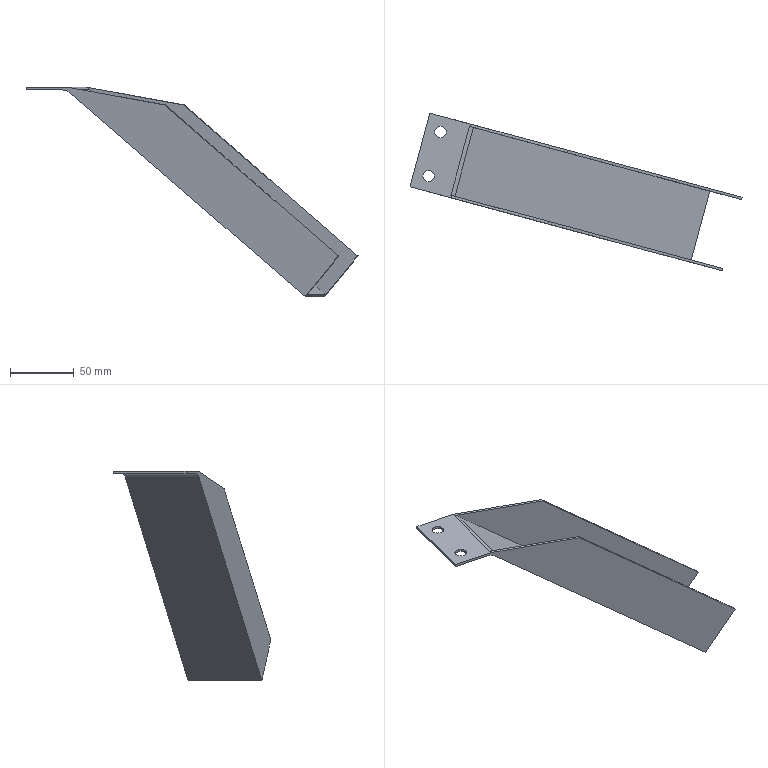Part | STEP file | lll_id3814_x_t | 1 solid | 18 faces | box 261.025 x 123.736 x 164.791 mm | volume 69372 mm3 | plane 14 | cylinder 4 | commonest cylinder face diameters 9 x2 20 x1 24 x1
STEP:
#1=CARTESIAN_POINT('',(375.612,286.459,-180.));
#2=VERTEX_POINT('',#1);
#3=CARTESIAN_POINT('',(452.222,265.931,-193.985));
#4=VERTEX_POINT('',#3);
#5=CARTESIAN_POINT('',(441.696,268.751,-192.064));
#6=DIRECTION('',(0.9513,-0.2549,-0.1736));
#7=VECTOR('',#6,1.);
#8=LINE('',#5,#7);
#9=EDGE_CURVE('',#2,#4,#8,.T.);
#10=ORIENTED_EDGE('',*,*,#9,.F.);
#11=CARTESIAN_POINT('',(375.094,284.527,-180.));
#12=VERTEX_POINT('',#11);
#13=CARTESIAN_POINT('',(295.378,-12.978,-180.));
#14=DIRECTION('',(0.2588,0.9659,0.));
#15=VECTOR('',#14,1.);
#16=LINE('',#13,#15);
#17=EDGE_CURVE('',#12,#2,#16,.T.);
#18=ORIENTED_EDGE('',*,*,#17,.F.);
#19=CARTESIAN_POINT('',(451.704,263.999,-193.985));
#20=VERTEX_POINT('',#19);
#21=CARTESIAN_POINT('',(441.179,266.819,-192.064));
#22=DIRECTION('',(0.9513,-0.2549,-0.1736));
#23=VECTOR('',#22,1.);
#24=LINE('',#21,#23);
#25=EDGE_CURVE('',#12,#20,#24,.T.);
#26=ORIENTED_EDGE('',*,*,#25,.T.);
#27=CARTESIAN_POINT('',(466.716,320.023,-193.985));
#28=DIRECTION('',(-0.2588,-0.9659,0.));
#29=VECTOR('',#28,1.);
#30=LINE('',#27,#29);
#31=EDGE_CURVE('',#4,#20,#30,.T.);
#32=ORIENTED_EDGE('',*,*,#31,.F.);
#33=EDGE_LOOP('',(#10,#18,#26,#32));
#34=FACE_OUTER_BOUND('',#33,.T.);
#35=CARTESIAN_POINT('',(232.191,3.953,-168.465));
#36=DIRECTION('',(0.1677,-0.04494,0.9848));
#37=DIRECTION('',(0.9513,-0.2549,-0.1736));
#38=AXIS2_PLACEMENT_3D('',#35,#36,#37);
#39=PLANE('',#38);
#40=ADVANCED_FACE('',(#34),#39,.T.);
#41=CARTESIAN_POINT('',(342.77,293.188,-180.));
#42=VERTEX_POINT('',#41);
#43=CARTESIAN_POINT('',(342.77,293.188,-182.));
#44=VERTEX_POINT('',#43);
#45=CARTESIAN_POINT('',(342.77,293.188,-180.));
#46=DIRECTION('',(0.,0.,-1.));
#47=VECTOR('',#46,1.);
#48=LINE('',#45,#47);
#49=EDGE_CURVE('',#42,#44,#48,.T.);
#50=ORIENTED_EDGE('',*,*,#49,.F.);
#51=CARTESIAN_POINT('',(358.3,351.143,-180.));
#52=VERTEX_POINT('',#51);
#53=CARTESIAN_POINT('',(358.3,351.143,-180.));
#54=DIRECTION('',(0.2588,0.9659,0.));
#55=VECTOR('',#54,1.);
#56=LINE('',#53,#55);
#57=EDGE_CURVE('',#42,#52,#56,.T.);
#58=ORIENTED_EDGE('',*,*,#57,.T.);
#59=CARTESIAN_POINT('',(358.3,351.143,-182.));
#60=VERTEX_POINT('',#59);
#61=CARTESIAN_POINT('',(358.3,351.143,-180.));
#62=DIRECTION('',(0.,0.,-1.));
#63=VECTOR('',#62,1.);
#64=LINE('',#61,#63);
#65=EDGE_CURVE('',#52,#60,#64,.T.);
#66=ORIENTED_EDGE('',*,*,#65,.T.);
#67=CARTESIAN_POINT('',(358.3,351.143,-182.));
#68=DIRECTION('',(0.2588,0.9659,0.));
#69=VECTOR('',#68,1.);
#70=LINE('',#67,#69);
#71=EDGE_CURVE('',#44,#60,#70,.T.);
#72=ORIENTED_EDGE('',*,*,#71,.F.);
#73=EDGE_LOOP('',(#50,#58,#66,#72));
#74=FACE_OUTER_BOUND('',#73,.T.);
#75=CARTESIAN_POINT('',(358.3,351.143,-180.));
#76=DIRECTION('',(0.9659,-0.2588,0.));
#77=DIRECTION('',(-0.2588,-0.9659,0.));
#78=AXIS2_PLACEMENT_3D('',#75,#76,#77);
#79=PLANE('',#78);
#80=ADVANCED_FACE('',(#74),#79,.F.);
#81=CARTESIAN_POINT('',(371.285,336.447,-180.));
#82=VERTEX_POINT('',#81);
#83=CARTESIAN_POINT('',(366.785,336.447,-180.));
#84=DIRECTION('',(0.,0.,1.));
#85=DIRECTION('',(1.,0.,0.));
#86=AXIS2_PLACEMENT_3D('',#83,#84,#85);
#87=CIRCLE('',#86,4.5);
#88=EDGE_CURVE('',#82,#82,#87,.T.);
#89=ORIENTED_EDGE('',*,*,#88,.T.);
#90=EDGE_LOOP('',(#89));
#91=FACE_BOUND('',#90,.T.);
#92=CARTESIAN_POINT('',(371.285,336.447,-182.));
#93=VERTEX_POINT('',#92);
#94=CARTESIAN_POINT('',(366.785,336.447,-182.));
#95=DIRECTION('',(0.,0.,1.));
#96=DIRECTION('',(1.,0.,0.));
#97=AXIS2_PLACEMENT_3D('',#94,#95,#96);
#98=CIRCLE('',#97,4.5);
#99=EDGE_CURVE('',#93,#93,#98,.T.);
#100=ORIENTED_EDGE('',*,*,#99,.F.);
#101=EDGE_LOOP('',(#100));
#102=FACE_BOUND('',#101,.T.);
#103=CARTESIAN_POINT('',(366.785,336.447,-182.));
#104=DIRECTION('',(0.,0.,1.));
#105=DIRECTION('',(1.,0.,0.));
#106=AXIS2_PLACEMENT_3D('',#103,#104,#105);
#107=CYLINDRICAL_SURFACE('',#106,4.5);
#108=ADVANCED_FACE('',(#91,#102),#107,.F.);
#109=CARTESIAN_POINT('',(361.967,301.673,-180.));
#110=VERTEX_POINT('',#109);
#111=CARTESIAN_POINT('',(357.467,301.673,-180.));
#112=DIRECTION('',(0.,0.,1.));
#113=DIRECTION('',(1.,0.,0.));
#114=AXIS2_PLACEMENT_3D('',#111,#112,#113);
#115=CIRCLE('',#114,4.5);
#116=EDGE_CURVE('',#110,#110,#115,.T.);
#117=ORIENTED_EDGE('',*,*,#116,.T.);
#118=EDGE_LOOP('',(#117));
#119=FACE_BOUND('',#118,.T.);
#120=CARTESIAN_POINT('',(361.967,301.673,-182.));
#121=VERTEX_POINT('',#120);
#122=CARTESIAN_POINT('',(357.467,301.673,-182.));
#123=DIRECTION('',(0.,0.,1.));
#124=DIRECTION('',(1.,0.,0.));
#125=AXIS2_PLACEMENT_3D('',#122,#123,#124);
#126=CIRCLE('',#125,4.5);
#127=EDGE_CURVE('',#121,#121,#126,.T.);
#128=ORIENTED_EDGE('',*,*,#127,.F.);
#129=EDGE_LOOP('',(#128));
#130=FACE_BOUND('',#129,.T.);
#131=CARTESIAN_POINT('',(357.467,301.673,-182.));
#132=DIRECTION('',(0.,0.,1.));
#133=DIRECTION('',(1.,0.,0.));
#134=AXIS2_PLACEMENT_3D('',#131,#132,#133);
#135=CYLINDRICAL_SURFACE('',#134,4.5);
#136=ADVANCED_FACE('',(#119,#130),#135,.F.);
#137=ORIENTED_EDGE('',*,*,#17,.T.);
#138=CARTESIAN_POINT('',(374.982,286.628,-180.));
#139=VERTEX_POINT('',#138);
#140=CARTESIAN_POINT('',(311.45,303.651,-180.));
#141=DIRECTION('',(-0.9659,0.2588,0.));
#142=VECTOR('',#141,1.);
#143=LINE('',#140,#142);
#144=EDGE_CURVE('',#2,#139,#143,.T.);
#145=ORIENTED_EDGE('',*,*,#144,.T.);
#146=CARTESIAN_POINT('',(389.476,340.719,-180.));
#147=VERTEX_POINT('',#146);
#148=CARTESIAN_POINT('',(382.229,313.673,-180.));
#149=DIRECTION('',(0.2588,0.9659,0.));
#150=VECTOR('',#149,1.);
#151=LINE('',#148,#150);
#152=EDGE_CURVE('',#139,#147,#151,.T.);
#153=ORIENTED_EDGE('',*,*,#152,.T.);
#154=CARTESIAN_POINT('',(390.106,340.55,-180.));
#155=VERTEX_POINT('',#154);
#156=CARTESIAN_POINT('',(530.346,302.973,-180.));
#157=DIRECTION('',(0.9659,-0.2588,0.));
#158=VECTOR('',#157,1.);
#159=LINE('',#156,#158);
#160=EDGE_CURVE('',#147,#155,#159,.T.);
#161=ORIENTED_EDGE('',*,*,#160,.T.);
#162=CARTESIAN_POINT('',(390.623,342.482,-180.));
#163=VERTEX_POINT('',#162);
#164=CARTESIAN_POINT('',(295.378,-12.978,-180.));
#165=DIRECTION('',(0.2588,0.9659,0.));
#166=VECTOR('',#165,1.);
#167=LINE('',#164,#166);
#168=EDGE_CURVE('',#155,#163,#167,.T.);
#169=ORIENTED_EDGE('',*,*,#168,.T.);
#170=CARTESIAN_POINT('',(549.109,300.016,-180.));
#171=DIRECTION('',(0.9659,-0.2588,0.));
#172=VECTOR('',#171,1.);
#173=LINE('',#170,#172);
#174=EDGE_CURVE('',#52,#163,#173,.T.);
#175=ORIENTED_EDGE('',*,*,#174,.F.);
#176=ORIENTED_EDGE('',*,*,#57,.F.);
#177=CARTESIAN_POINT('',(442.198,266.546,-180.));
#178=DIRECTION('',(0.9659,-0.2588,0.));
#179=VECTOR('',#178,1.);
#180=LINE('',#177,#179);
#181=EDGE_CURVE('',#42,#12,#180,.T.);
#182=ORIENTED_EDGE('',*,*,#181,.T.);
#183=EDGE_LOOP('',(#137,#145,#153,#161,#169,#175,#176,#182));
#184=FACE_BOUND('',#183,.T.);
#185=ORIENTED_EDGE('',*,*,#116,.F.);
#186=EDGE_LOOP('',(#185));
#187=FACE_BOUND('',#186,.T.);
#188=ORIENTED_EDGE('',*,*,#88,.F.);
#189=EDGE_LOOP('',(#188));
#190=FACE_BOUND('',#189,.T.);
#191=CARTESIAN_POINT('',(231.216,4.214,-180.));
#192=DIRECTION('',(0.,0.,1.));
#193=DIRECTION('',(0.9659,-0.2588,0.));
#194=AXIS2_PLACEMENT_3D('',#191,#192,#193);
#195=PLANE('',#194);
#196=ADVANCED_FACE('',(#184,#187,#190),#195,.T.);
#197=CARTESIAN_POINT('',(386.104,343.693,-182.));
#198=VERTEX_POINT('',#197);
#199=CARTESIAN_POINT('',(387.277,343.379,-182.));
#200=DIRECTION('',(0.9659,-0.2588,0.));
#201=VECTOR('',#200,1.);
#202=LINE('',#199,#201);
#203=EDGE_CURVE('',#60,#198,#202,.T.);
#204=ORIENTED_EDGE('',*,*,#203,.T.);
#205=CARTESIAN_POINT('',(370.575,285.738,-182.));
#206=VERTEX_POINT('',#205);
#207=CARTESIAN_POINT('',(370.575,285.738,-182.));
#208=DIRECTION('',(-0.2588,-0.9659,0.));
#209=VECTOR('',#208,1.);
#210=LINE('',#207,#209);
#211=EDGE_CURVE('',#198,#206,#210,.T.);
#212=ORIENTED_EDGE('',*,*,#211,.T.);
#213=CARTESIAN_POINT('',(371.748,285.423,-182.));
#214=DIRECTION('',(-0.9659,0.2588,0.));
#215=VECTOR('',#214,1.);
#216=LINE('',#213,#215);
#217=EDGE_CURVE('',#206,#44,#216,.T.);
#218=ORIENTED_EDGE('',*,*,#217,.T.);
#219=ORIENTED_EDGE('',*,*,#71,.T.);
#220=EDGE_LOOP('',(#204,#212,#218,#219));
#221=FACE_BOUND('',#220,.T.);
#222=ORIENTED_EDGE('',*,*,#127,.T.);
#223=EDGE_LOOP('',(#222));
#224=FACE_BOUND('',#223,.T.);
#225=ORIENTED_EDGE('',*,*,#99,.T.);
#226=EDGE_LOOP('',(#225));
#227=FACE_BOUND('',#226,.T.);
#228=CARTESIAN_POINT('',(387.277,343.379,-182.));
#229=DIRECTION('',(0.,0.,-1.));
#230=DIRECTION('',(-1.,0.,0.));
#231=AXIS2_PLACEMENT_3D('',#228,#229,#230);
#232=PLANE('',#231);
#233=ADVANCED_FACE('',(#221,#224,#227),#232,.T.);
#234=ORIENTED_EDGE('',*,*,#217,.F.);
#235=CARTESIAN_POINT('',(378.026,283.741,-184.807));
#236=VERTEX_POINT('',#235);
#237=CARTESIAN_POINT('',(370.575,285.738,-194.));
#238=DIRECTION('',(0.2588,0.9659,0.));
#239=DIRECTION('',(-0.9659,0.2588,0.));
#240=AXIS2_PLACEMENT_3D('',#237,#238,#239);
#241=CIRCLE('',#240,12.);
#242=EDGE_CURVE('',#206,#236,#241,.T.);
#243=ORIENTED_EDGE('',*,*,#242,.T.);
#244=CARTESIAN_POINT('',(562.189,234.395,-344.791));
#245=VERTEX_POINT('',#244);
#246=CARTESIAN_POINT('',(514.093,247.282,-303.009));
#247=DIRECTION('',(0.7399,-0.1983,-0.6428));
#248=VECTOR('',#247,1.);
#249=LINE('',#246,#248);
#250=EDGE_CURVE('',#236,#245,#249,.T.);
#251=ORIENTED_EDGE('',*,*,#250,.T.);
#252=CARTESIAN_POINT('',(588.267,227.407,-312.617));
#253=VERTEX_POINT('',#252);
#254=CARTESIAN_POINT('',(563.431,234.062,-343.259));
#255=DIRECTION('',(0.6209,-0.1664,0.766));
#256=VECTOR('',#255,1.);
#257=LINE('',#254,#256);
#258=EDGE_CURVE('',#245,#253,#257,.T.);
#259=ORIENTED_EDGE('',*,*,#258,.T.);
#260=CARTESIAN_POINT('',(462.863,261.009,-203.679));
#261=DIRECTION('',(0.7399,-0.1983,-0.6428));
#262=VECTOR('',#261,1.);
#263=LINE('',#260,#262);
#264=EDGE_CURVE('',#20,#253,#263,.T.);
#265=ORIENTED_EDGE('',*,*,#264,.F.);
#266=ORIENTED_EDGE('',*,*,#25,.F.);
#267=ORIENTED_EDGE('',*,*,#181,.F.);
#268=ORIENTED_EDGE('',*,*,#49,.T.);
#269=EDGE_LOOP('',(#234,#243,#251,#259,#265,#266,#267,#268));
#270=FACE_OUTER_BOUND('',#269,.T.);
#271=CARTESIAN_POINT('',(442.198,266.546,-229.326));
#272=DIRECTION('',(0.2588,0.9659,0.));
#273=DIRECTION('',(0.,0.,1.));
#274=AXIS2_PLACEMENT_3D('',#271,#272,#273);
#275=PLANE('',#274);
#276=ADVANCED_FACE('',(#270),#275,.F.);
#277=ORIENTED_EDGE('',*,*,#174,.T.);
#278=CARTESIAN_POINT('',(467.233,321.955,-193.985));
#279=VERTEX_POINT('',#278);
#280=CARTESIAN_POINT('',(546.701,300.661,-208.492));
#281=DIRECTION('',(0.9513,-0.2549,-0.1736));
#282=VECTOR('',#281,1.);
#283=LINE('',#280,#282);
#284=EDGE_CURVE('',#163,#279,#283,.T.);
#285=ORIENTED_EDGE('',*,*,#284,.T.);
#286=CARTESIAN_POINT('',(603.796,285.363,-312.617));
#287=VERTEX_POINT('',#286);
#288=CARTESIAN_POINT('',(555.7,298.25,-270.836));
#289=DIRECTION('',(-0.7399,0.1983,0.6428));
#290=VECTOR('',#289,1.);
#291=LINE('',#288,#290);
#292=EDGE_CURVE('',#287,#279,#291,.T.);
#293=ORIENTED_EDGE('',*,*,#292,.F.);
#294=CARTESIAN_POINT('',(577.719,292.35,-344.791));
#295=VERTEX_POINT('',#294);
#296=CARTESIAN_POINT('',(578.96,292.018,-343.259));
#297=DIRECTION('',(-0.6209,0.1664,-0.766));
#298=VECTOR('',#297,1.);
#299=LINE('',#296,#298);
#300=EDGE_CURVE('',#287,#295,#299,.T.);
#301=ORIENTED_EDGE('',*,*,#300,.T.);
#302=CARTESIAN_POINT('',(393.555,341.697,-184.807));
#303=VERTEX_POINT('',#302);
#304=CARTESIAN_POINT('',(529.622,305.238,-303.009));
#305=DIRECTION('',(-0.7399,0.1983,0.6428));
#306=VECTOR('',#305,1.);
#307=LINE('',#304,#306);
#308=EDGE_CURVE('',#295,#303,#307,.T.);
#309=ORIENTED_EDGE('',*,*,#308,.T.);
#310=CARTESIAN_POINT('',(386.104,343.693,-194.));
#311=DIRECTION('',(-0.2588,-0.9659,0.));
#312=DIRECTION('',(-0.9659,0.2588,0.));
#313=AXIS2_PLACEMENT_3D('',#310,#311,#312);
#314=CIRCLE('',#313,12.);
#315=EDGE_CURVE('',#303,#198,#314,.T.);
#316=ORIENTED_EDGE('',*,*,#315,.T.);
#317=ORIENTED_EDGE('',*,*,#203,.F.);
#318=ORIENTED_EDGE('',*,*,#65,.F.);
#319=EDGE_LOOP('',(#277,#285,#293,#301,#309,#316,#317,#318));
#320=FACE_OUTER_BOUND('',#319,.T.);
#321=CARTESIAN_POINT('',(549.109,300.016,-274.42));
#322=DIRECTION('',(0.2588,0.9659,0.));
#323=DIRECTION('',(-0.8365,0.2241,0.5));
#324=AXIS2_PLACEMENT_3D('',#321,#322,#323);
#325=PLANE('',#324);
#326=ADVANCED_FACE('',(#320),#325,.T.);
#327=ORIENTED_EDGE('',*,*,#168,.F.);
#328=CARTESIAN_POINT('',(466.716,320.023,-193.985));
#329=VERTEX_POINT('',#328);
#330=CARTESIAN_POINT('',(546.184,298.73,-208.492));
#331=DIRECTION('',(0.9513,-0.2549,-0.1736));
#332=VECTOR('',#331,1.);
#333=LINE('',#330,#332);
#334=EDGE_CURVE('',#155,#329,#333,.T.);
#335=ORIENTED_EDGE('',*,*,#334,.T.);
#336=CARTESIAN_POINT('',(466.716,320.023,-193.985));
#337=DIRECTION('',(-0.2588,-0.9659,0.));
#338=VECTOR('',#337,1.);
#339=LINE('',#336,#338);
#340=EDGE_CURVE('',#279,#329,#339,.T.);
#341=ORIENTED_EDGE('',*,*,#340,.F.);
#342=ORIENTED_EDGE('',*,*,#284,.F.);
#343=EDGE_LOOP('',(#327,#335,#341,#342));
#344=FACE_OUTER_BOUND('',#343,.T.);
#345=CARTESIAN_POINT('',(232.191,3.953,-168.465));
#346=DIRECTION('',(0.1677,-0.04494,0.9848));
#347=DIRECTION('',(0.9513,-0.2549,-0.1736));
#348=AXIS2_PLACEMENT_3D('',#345,#346,#347);
#349=PLANE('',#348);
#350=ADVANCED_FACE('',(#344),#349,.T.);
#351=CARTESIAN_POINT('',(578.443,290.086,-343.259));
#352=VERTEX_POINT('',#351);
#353=CARTESIAN_POINT('',(392.598,339.883,-181.815));
#354=VERTEX_POINT('',#353);
#355=CARTESIAN_POINT('',(530.346,302.973,-301.477));
#356=DIRECTION('',(-0.7399,0.1983,0.6428));
#357=VECTOR('',#356,1.);
#358=LINE('',#355,#357);
#359=EDGE_CURVE('',#352,#354,#358,.T.);
#360=ORIENTED_EDGE('',*,*,#359,.T.);
#361=CARTESIAN_POINT('',(378.104,285.791,-181.815));
#362=VERTEX_POINT('',#361);
#363=CARTESIAN_POINT('',(346.011,166.016,-181.815));
#364=DIRECTION('',(-0.2588,-0.9659,0.));
#365=VECTOR('',#364,1.);
#366=LINE('',#363,#365);
#367=EDGE_CURVE('',#354,#362,#366,.T.);
#368=ORIENTED_EDGE('',*,*,#367,.T.);
#369=CARTESIAN_POINT('',(563.949,235.994,-343.259));
#370=VERTEX_POINT('',#369);
#371=CARTESIAN_POINT('',(515.853,248.881,-301.477));
#372=DIRECTION('',(0.7399,-0.1983,-0.6428));
#373=VECTOR('',#372,1.);
#374=LINE('',#371,#373);
#375=EDGE_CURVE('',#362,#370,#374,.T.);
#376=ORIENTED_EDGE('',*,*,#375,.T.);
#377=CARTESIAN_POINT('',(531.855,116.219,-343.259));
#378=DIRECTION('',(0.2588,0.9659,0.));
#379=VECTOR('',#378,1.);
#380=LINE('',#377,#379);
#381=EDGE_CURVE('',#370,#352,#380,.T.);
#382=ORIENTED_EDGE('',*,*,#381,.T.);
#383=EDGE_LOOP('',(#360,#368,#376,#382));
#384=FACE_OUTER_BOUND('',#383,.T.);
#385=CARTESIAN_POINT('',(483.759,129.106,-301.477));
#386=DIRECTION('',(-0.6209,0.1664,-0.766));
#387=DIRECTION('',(-0.7399,0.1983,0.6428));
#388=AXIS2_PLACEMENT_3D('',#385,#386,#387);
#389=PLANE('',#388);
#390=ADVANCED_FACE('',(#384),#389,.F.);
#391=ORIENTED_EDGE('',*,*,#250,.F.);
#392=CARTESIAN_POINT('',(393.555,341.697,-184.807));
#393=DIRECTION('',(0.2588,0.9659,0.));
#394=VECTOR('',#393,1.);
#395=LINE('',#392,#394);
#396=EDGE_CURVE('',#236,#303,#395,.T.);
#397=ORIENTED_EDGE('',*,*,#396,.T.);
#398=ORIENTED_EDGE('',*,*,#308,.F.);
#399=CARTESIAN_POINT('',(530.614,116.552,-344.791));
#400=DIRECTION('',(0.2588,0.9659,0.));
#401=VECTOR('',#400,1.);
#402=LINE('',#399,#401);
#403=EDGE_CURVE('',#245,#295,#402,.T.);
#404=ORIENTED_EDGE('',*,*,#403,.F.);
#405=EDGE_LOOP('',(#391,#397,#398,#404));
#406=FACE_OUTER_BOUND('',#405,.T.);
#407=CARTESIAN_POINT('',(482.517,129.439,-303.009));
#408=DIRECTION('',(-0.6209,0.1664,-0.766));
#409=DIRECTION('',(-0.7399,0.1983,0.6428));
#410=AXIS2_PLACEMENT_3D('',#407,#408,#409);
#411=PLANE('',#410);
#412=ADVANCED_FACE('',(#406),#411,.T.);
#413=ORIENTED_EDGE('',*,*,#334,.F.);
#414=ORIENTED_EDGE('',*,*,#160,.F.);
#415=CARTESIAN_POINT('',(386.389,341.546,-189.476));
#416=DIRECTION('',(0.2588,0.9659,0.));
#417=DIRECTION('',(-0.9659,0.2588,0.));
#418=AXIS2_PLACEMENT_3D('',#415,#416,#417);
#419=CIRCLE('',#418,10.);
#420=EDGE_CURVE('',#147,#354,#419,.T.);
#421=ORIENTED_EDGE('',*,*,#420,.T.);
#422=ORIENTED_EDGE('',*,*,#359,.F.);
#423=CARTESIAN_POINT('',(603.278,283.431,-312.617));
#424=VERTEX_POINT('',#423);
#425=CARTESIAN_POINT('',(578.443,290.086,-343.259));
#426=DIRECTION('',(-0.6209,0.1664,-0.766));
#427=VECTOR('',#426,1.);
#428=LINE('',#425,#427);
#429=EDGE_CURVE('',#424,#352,#428,.T.);
#430=ORIENTED_EDGE('',*,*,#429,.F.);
#431=CARTESIAN_POINT('',(555.182,296.318,-270.836));
#432=DIRECTION('',(-0.7399,0.1983,0.6428));
#433=VECTOR('',#432,1.);
#434=LINE('',#431,#433);
#435=EDGE_CURVE('',#424,#329,#434,.T.);
#436=ORIENTED_EDGE('',*,*,#435,.T.);
#437=EDGE_LOOP('',(#413,#414,#421,#422,#430,#436));
#438=FACE_OUTER_BOUND('',#437,.T.);
#439=CARTESIAN_POINT('',(530.346,302.973,-301.477));
#440=DIRECTION('',(0.2588,0.9659,0.));
#441=DIRECTION('',(-0.7399,0.1983,0.6428));
#442=AXIS2_PLACEMENT_3D('',#439,#440,#441);
#443=PLANE('',#442);
#444=ADVANCED_FACE('',(#438),#443,.F.);
#445=ORIENTED_EDGE('',*,*,#292,.T.);
#446=ORIENTED_EDGE('',*,*,#340,.T.);
#447=ORIENTED_EDGE('',*,*,#435,.F.);
#448=CARTESIAN_POINT('',(603.278,283.431,-312.617));
#449=DIRECTION('',(0.2588,0.9659,0.));
#450=VECTOR('',#449,1.);
#451=LINE('',#448,#450);
#452=EDGE_CURVE('',#424,#287,#451,.T.);
#453=ORIENTED_EDGE('',*,*,#452,.T.);
#454=EDGE_LOOP('',(#445,#446,#447,#453));
#455=FACE_OUTER_BOUND('',#454,.T.);
#456=CARTESIAN_POINT('',(555.182,296.318,-270.836));
#457=DIRECTION('',(-0.6209,0.1664,-0.766));
#458=DIRECTION('',(-0.7399,0.1983,0.6428));
#459=AXIS2_PLACEMENT_3D('',#456,#457,#458);
#460=PLANE('',#459);
#461=ADVANCED_FACE('',(#455),#460,.F.);
#462=ORIENTED_EDGE('',*,*,#375,.F.);
#463=CARTESIAN_POINT('',(371.895,287.454,-189.476));
#464=DIRECTION('',(-0.2588,-0.9659,0.));
#465=DIRECTION('',(-0.9659,0.2588,0.));
#466=AXIS2_PLACEMENT_3D('',#463,#464,#465);
#467=CIRCLE('',#466,10.);
#468=EDGE_CURVE('',#362,#139,#467,.T.);
#469=ORIENTED_EDGE('',*,*,#468,.T.);
#470=ORIENTED_EDGE('',*,*,#144,.F.);
#471=ORIENTED_EDGE('',*,*,#9,.T.);
#472=CARTESIAN_POINT('',(588.784,229.339,-312.617));
#473=VERTEX_POINT('',#472);
#474=CARTESIAN_POINT('',(463.381,262.941,-203.679));
#475=DIRECTION('',(0.7399,-0.1983,-0.6428));
#476=VECTOR('',#475,1.);
#477=LINE('',#474,#476);
#478=EDGE_CURVE('',#4,#473,#477,.T.);
#479=ORIENTED_EDGE('',*,*,#478,.T.);
#480=CARTESIAN_POINT('',(563.949,235.994,-343.259));
#481=DIRECTION('',(0.6209,-0.1664,0.766));
#482=VECTOR('',#481,1.);
#483=LINE('',#480,#482);
#484=EDGE_CURVE('',#370,#473,#483,.T.);
#485=ORIENTED_EDGE('',*,*,#484,.F.);
#486=EDGE_LOOP('',(#462,#469,#470,#471,#479,#485));
#487=FACE_OUTER_BOUND('',#486,.T.);
#488=CARTESIAN_POINT('',(433.423,270.968,-240.64));
#489=DIRECTION('',(0.2588,0.9659,0.));
#490=DIRECTION('',(0.1677,-0.04494,0.9848));
#491=AXIS2_PLACEMENT_3D('',#488,#489,#490);
#492=PLANE('',#491);
#493=ADVANCED_FACE('',(#487),#492,.T.);
#494=ORIENTED_EDGE('',*,*,#478,.F.);
#495=ORIENTED_EDGE('',*,*,#31,.T.);
#496=ORIENTED_EDGE('',*,*,#264,.T.);
#497=CARTESIAN_POINT('',(556.691,109.564,-312.617));
#498=DIRECTION('',(-0.2588,-0.9659,0.));
#499=VECTOR('',#498,1.);
#500=LINE('',#497,#499);
#501=EDGE_CURVE('',#473,#253,#500,.T.);
#502=ORIENTED_EDGE('',*,*,#501,.F.);
#503=EDGE_LOOP('',(#494,#495,#496,#502));
#504=FACE_OUTER_BOUND('',#503,.T.);
#505=CARTESIAN_POINT('',(555.182,296.318,-270.836));
#506=DIRECTION('',(-0.6209,0.1664,-0.766));
#507=DIRECTION('',(-0.7399,0.1983,0.6428));
#508=AXIS2_PLACEMENT_3D('',#505,#506,#507);
#509=PLANE('',#508);
#510=ADVANCED_FACE('',(#504),#509,.F.);
#511=ORIENTED_EDGE('',*,*,#381,.F.);
#512=ORIENTED_EDGE('',*,*,#484,.T.);
#513=ORIENTED_EDGE('',*,*,#501,.T.);
#514=ORIENTED_EDGE('',*,*,#258,.F.);
#515=ORIENTED_EDGE('',*,*,#403,.T.);
#516=ORIENTED_EDGE('',*,*,#300,.F.);
#517=ORIENTED_EDGE('',*,*,#452,.F.);
#518=ORIENTED_EDGE('',*,*,#429,.T.);
#519=EDGE_LOOP('',(#511,#512,#513,#514,#515,#516,#517,#518));
#520=FACE_OUTER_BOUND('',#519,.T.);
#521=CARTESIAN_POINT('',(531.855,116.219,-343.259));
#522=DIRECTION('',(0.7399,-0.1983,-0.6428));
#523=DIRECTION('',(-0.6209,0.1664,-0.766));
#524=AXIS2_PLACEMENT_3D('',#521,#522,#523);
#525=PLANE('',#524);
#526=ADVANCED_FACE('',(#520),#525,.T.);
#527=ORIENTED_EDGE('',*,*,#420,.F.);
#528=ORIENTED_EDGE('',*,*,#152,.F.);
#529=ORIENTED_EDGE('',*,*,#468,.F.);
#530=ORIENTED_EDGE('',*,*,#367,.F.);
#531=EDGE_LOOP('',(#527,#528,#529,#530));
#532=FACE_OUTER_BOUND('',#531,.T.);
#533=CARTESIAN_POINT('',(339.802,167.68,-189.476));
#534=DIRECTION('',(0.2588,0.9659,0.));
#535=DIRECTION('',(-0.9659,0.2588,0.));
#536=AXIS2_PLACEMENT_3D('',#533,#534,#535);
#537=CYLINDRICAL_SURFACE('',#536,10.);
#538=ADVANCED_FACE('',(#532),#537,.T.);
#539=ORIENTED_EDGE('',*,*,#242,.F.);
#540=ORIENTED_EDGE('',*,*,#211,.F.);
#541=ORIENTED_EDGE('',*,*,#315,.F.);
#542=ORIENTED_EDGE('',*,*,#396,.F.);
#543=EDGE_LOOP('',(#539,#540,#541,#542));
#544=FACE_OUTER_BOUND('',#543,.T.);
#545=CARTESIAN_POINT('',(338.999,167.895,-194.));
#546=DIRECTION('',(-0.2588,-0.9659,0.));
#547=DIRECTION('',(0.9659,-0.2588,0.));
#548=AXIS2_PLACEMENT_3D('',#545,#546,#547);
#549=CYLINDRICAL_SURFACE('',#548,12.);
#550=ADVANCED_FACE('',(#544),#549,.F.);
#551=CLOSED_SHELL('',(#40,#80,#108,#136,#196,#233,#276,#326,#350,#390,#412,#444,#461,#493,#510,#526,#538,#550));
#552=MANIFOLD_SOLID_BREP('',#551);
#553=(LENGTH_UNIT()NAMED_UNIT(*)SI_UNIT(.MILLI.,.METRE.));
#554=UNCERTAINTY_MEASURE_WITH_UNIT(LENGTH_MEASURE(0.00002),#553,'','');
#555=(NAMED_UNIT(*)PLANE_ANGLE_UNIT()SI_UNIT($,.RADIAN.));
#556=PLANE_ANGLE_MEASURE_WITH_UNIT(PLANE_ANGLE_MEASURE(0.01745),#555);
#557=DIMENSIONAL_EXPONENTS(0.,0.,0.,0.,0.,0.,0.);
#558=(CONVERSION_BASED_UNIT('DEGREE',#556)NAMED_UNIT(#557)PLANE_ANGLE_UNIT());
#559=(NAMED_UNIT(*)SI_UNIT($,.STERADIAN.)SOLID_ANGLE_UNIT());
#560=(GEOMETRIC_REPRESENTATION_CONTEXT(3)GLOBAL_UNCERTAINTY_ASSIGNED_CONTEXT((#554))GLOBAL_UNIT_ASSIGNED_CONTEXT((#553,#558,#559))REPRESENTATION_CONTEXT('',''));
#561=ADVANCED_BREP_SHAPE_REPRESENTATION('',(#552),#560);